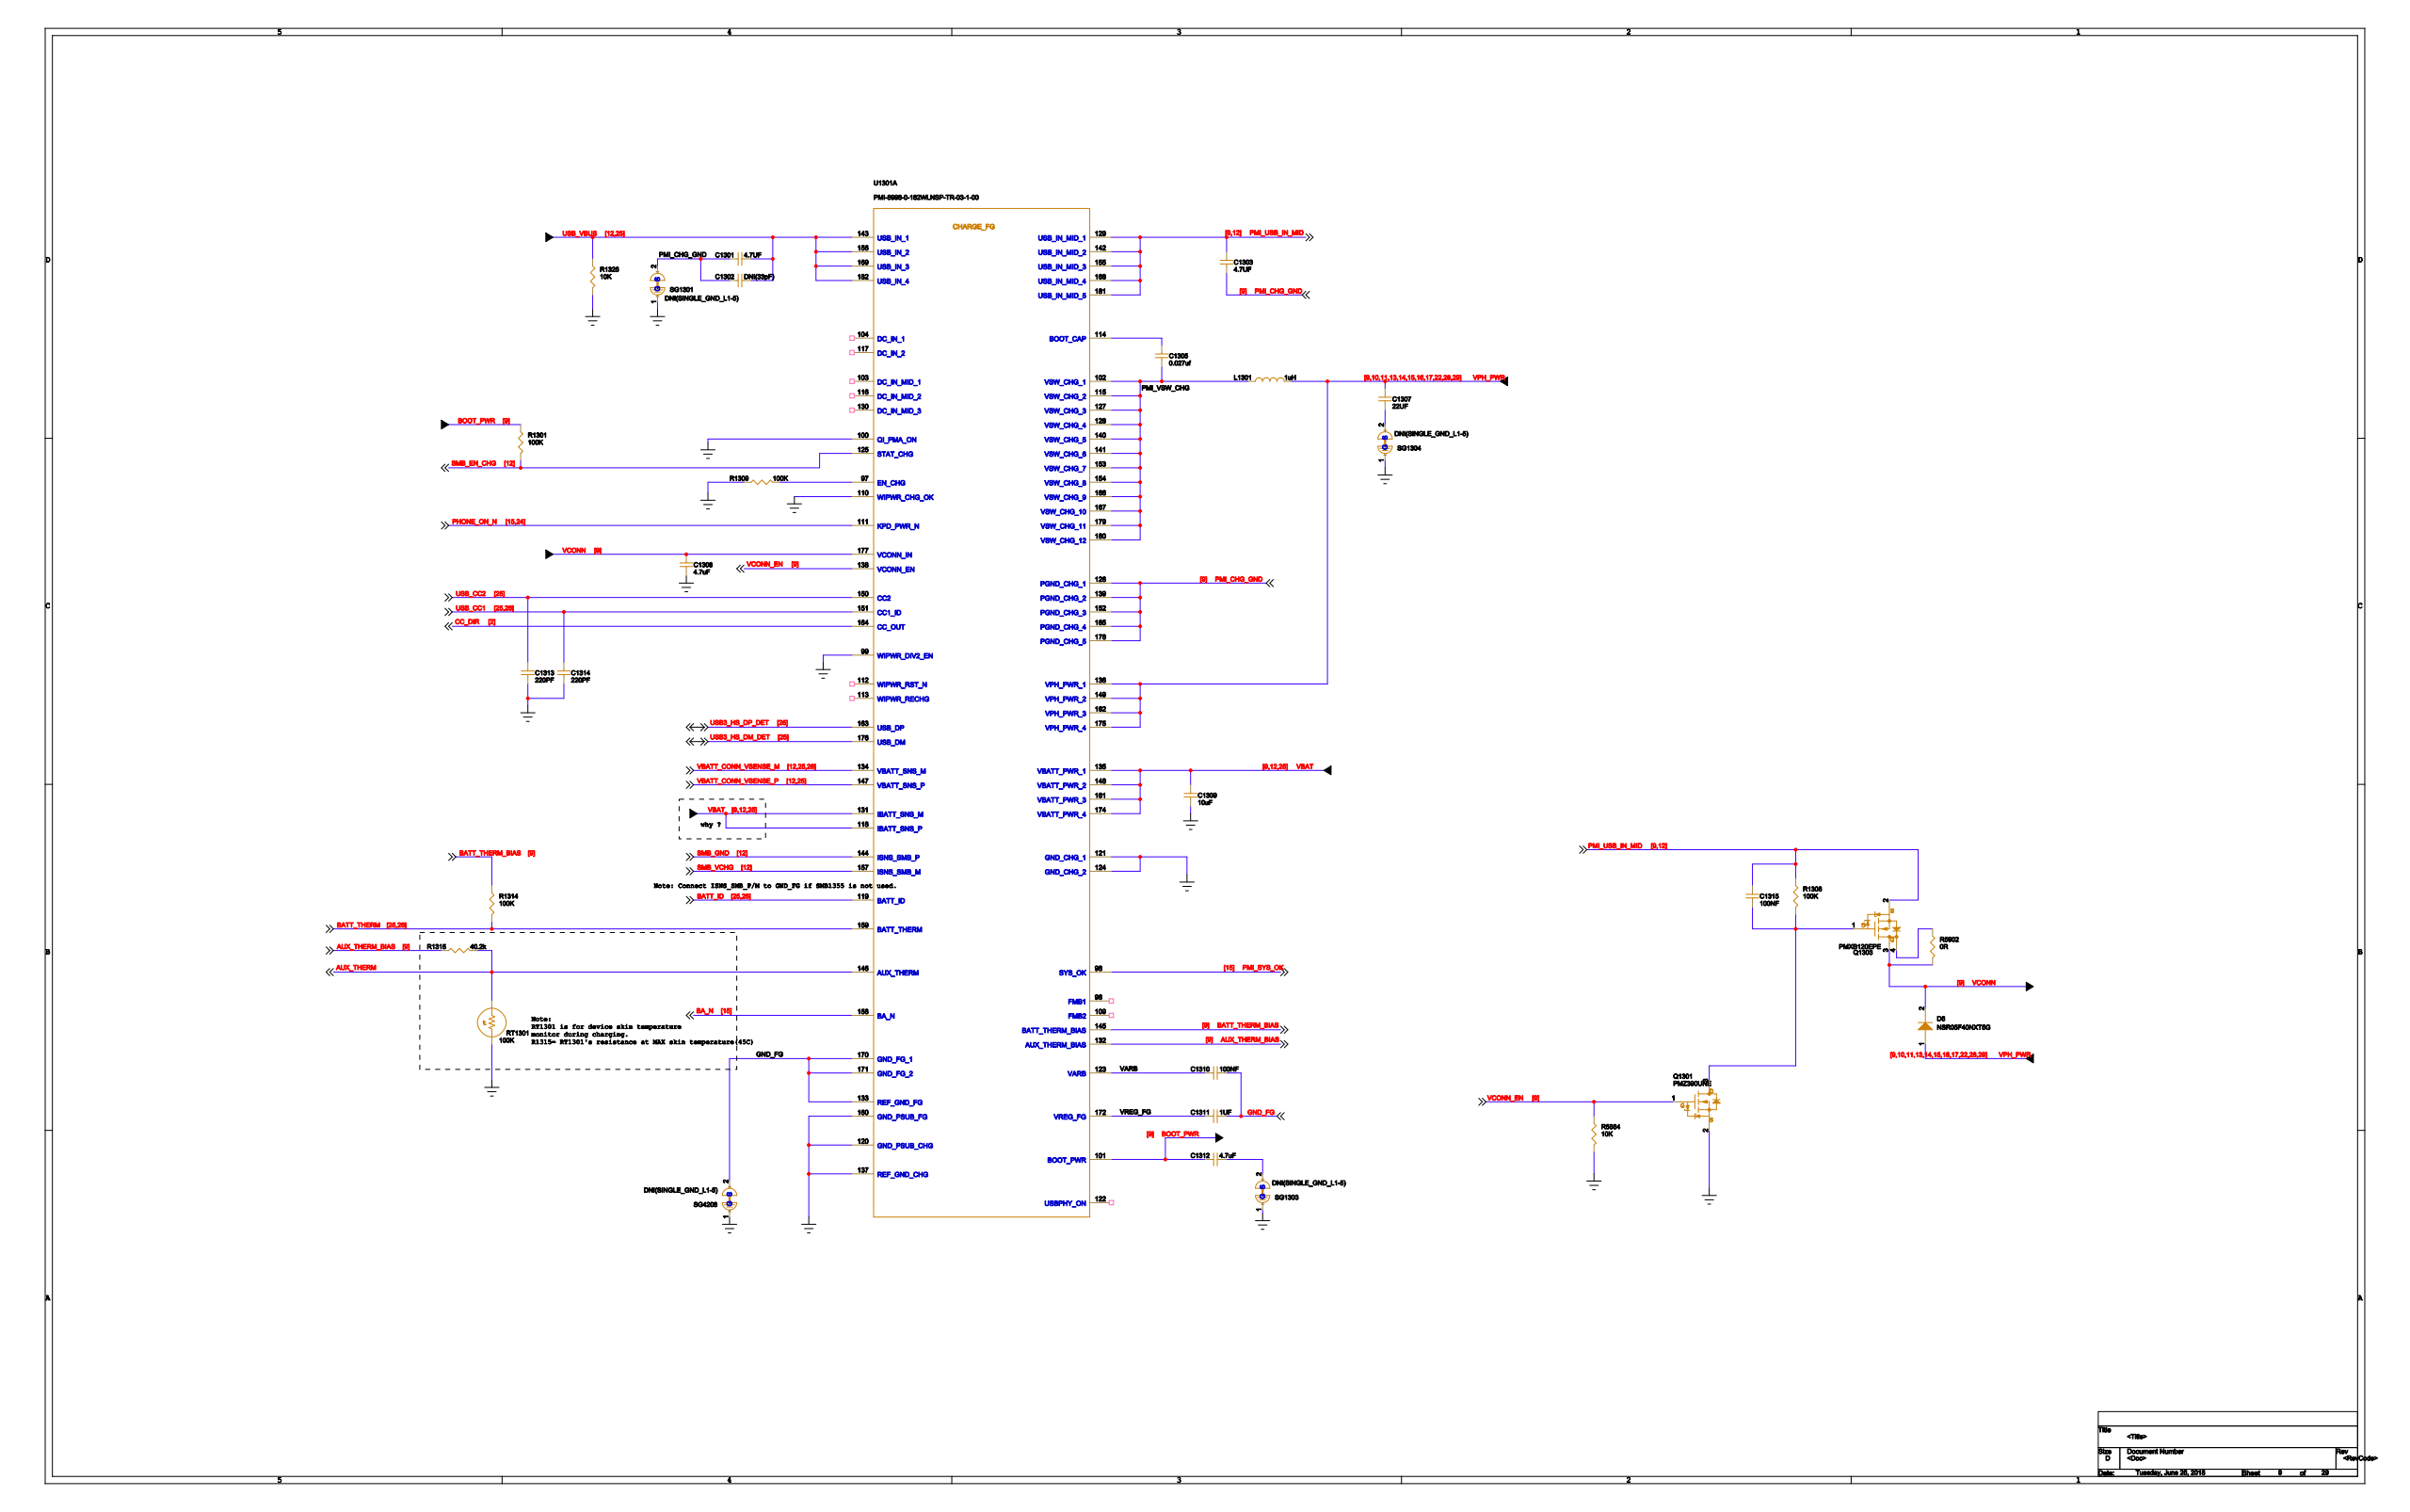Circuit board | Cadence Allegro | 802 parts | 566 nets | one sheet of the schematic
Parts on this sheet (reference | value | footprint):
C1301 | 4.7UF | 0603-BIG
C1302 | DNI(33pF) | C0201
C1303 | 4.7UF | 0603-BIG
C1305 | 0.027uf | 0402-BIG
C1307 | 22UF | 0603-BIG
C1308 | 4.7uF | 0402-BIG
C1309 | 10uF | 0402-BIG
C1310 | 100NF | C0201
C1311 | 1uF | C0201
C1312 | 4.7uF | 0402-BIG
C1313 | 220PF | C0201
C1314 | 220PF | C0201
C1315 | 100NF | C0201
D6 | NSR05F40NXT5G | DSN2
L1301 | 1uH | L2520_MEKK2520
Q1301 | PMZ390UNE | SOT883_PMZ390UN
Q1303 | PMXB120EPE | PMXB120EPE
R1301 | 100K | R0201
R1308 | 100K | R0201
R1309 | 100K | R0201
R1314 | 100K | R0201
R1315 | 40.2k | R0201
R1326 | 10K | R0201
R5884 | 10K | R0402
R5902 | 0R | R0201
RT1301 | 100K | R0402
SG1301 | DNI(SINGLE_GND_L1-5) | GND_L1-5
SG1303 | DNI(SINGLE_GND_L1-5) | GND_L1-5
SG1304 | DNI(SINGLE_GND_L1-5) | GND_L1-5
SG4208 | DNI(SINGLE_GND_L1-5) | GND_L1-5
U1301 | PMI-8998-0-182WLNSP-TR-03-1-00 | PMI8998
Nets of these parts (net: part-pin ...):
GND: C1308-2 C1309-2 C1313-2 C1314-2 Q1301-2 R1309-1 R1326-2 R5884-2 RT1301-2 SG1301-1 SG1303-1 SG1304-1 SG4208-1 U1301-3 U1301-4 U1301-15 U1301-99 U1301-100 U1301-110 U1301-120 U1301-121 U1301-124 U1301-137 U1301-160
VBATT_CONN_VSENSE_P: U1301-147
BATT_ID: U1301-119
VBATT_CONN_VSENSE_M: U1301-134
BATT_THERM: R1314-2 U1301-159
VBAT: C1309-1 U1301-118 U1301-131 U1301-135 U1301-148 U1301-161 U1301-174
PMI_CHG_GND: C1301-1 C1302-1 C1303-2 SG1301-2 U1301-126 U1301-139 U1301-152 U1301-165 U1301-178
USB_VBUS: C1301-2 C1302-2 R1326-1 U1301-143 U1301-156 U1301-169 U1301-182
VPH_PWR: C1307-1 D6-1 L1301-2 U1301-2 U1301-9 U1301-22 U1301-136 U1301-149 U1301-162 U1301-175
VARB: C1310-1 U1301-123
GND_FG: C1310-2 C1311-2 SG4208-2 U1301-133 U1301-170 U1301-171
PMI_USB_IN_MID: C1303-1 C1315-1 Q1303-2 R1308-1 U1301-129 U1301-142 U1301-155 U1301-168 U1301-181
N366823: C1315-2 Q1301-3 Q1303-1 R1308-2
VCONN: C1308-1 D6-2 Q1303-3 R5902-2 U1301-177
N1009370: Q1303-4 R5902-1
VREG_FG: C1311-1 U1301-172
USB_CC1: C1314-1 U1301-151
USB_CC2: C1313-1 U1301-150
VCONN_EN: Q1301-1 R5884-1 U1301-138
N147788: C1305-1 U1301-114
PMI_VSW_CHG: C1305-2 L1301-1 U1301-102 U1301-115 U1301-127 U1301-128 U1301-140 U1301-141 U1301-153 U1301-154 U1301-166 U1301-167 U1301-179 U1301-180
N147824: C1307-2 SG1304-2
BOOT_PWR: C1312-1 R1301-1 U1301-101
N147670: C1312-2 SG1303-2
USB3_HS_DM_DET: U1301-176
USB3_HS_DP_DET: U1301-163
BATT_THERM_BIAS: R1314-1 U1301-145
SMB_EN_CHG: R1301-2 U1301-125
N147488: R1309-2 U1301-97
AUX_THERM_BIAS: R1315-1 U1301-132
AUX_THERM: R1315-2 RT1301-1 U1301-146
PHONE_ON_N: U1301-111
SMB_GND: U1301-144
BA_N: U1301-158
CC_DIR: U1301-164
SMB_VCHG: U1301-157
PMI_SYS_OK: U1301-98